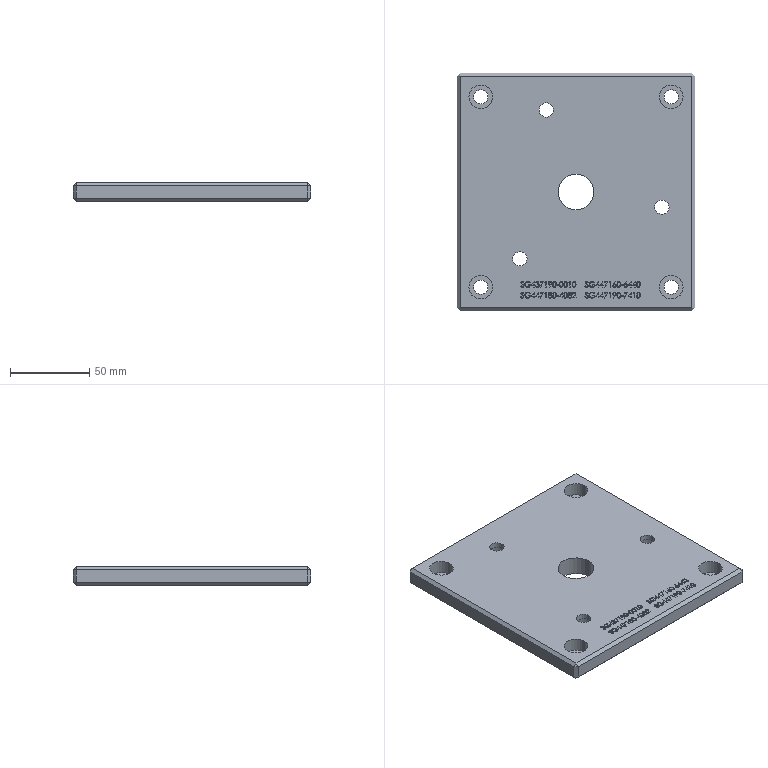Part | STEP file | Shim select base | 1 solid | 690 faces | box 150 x 150 x 12 mm | volume 250622 mm3 | plane 384 | spline 276 | cylinder 30 | commonest cylinder face diameters 9 x14 15 x14 22.5 x2